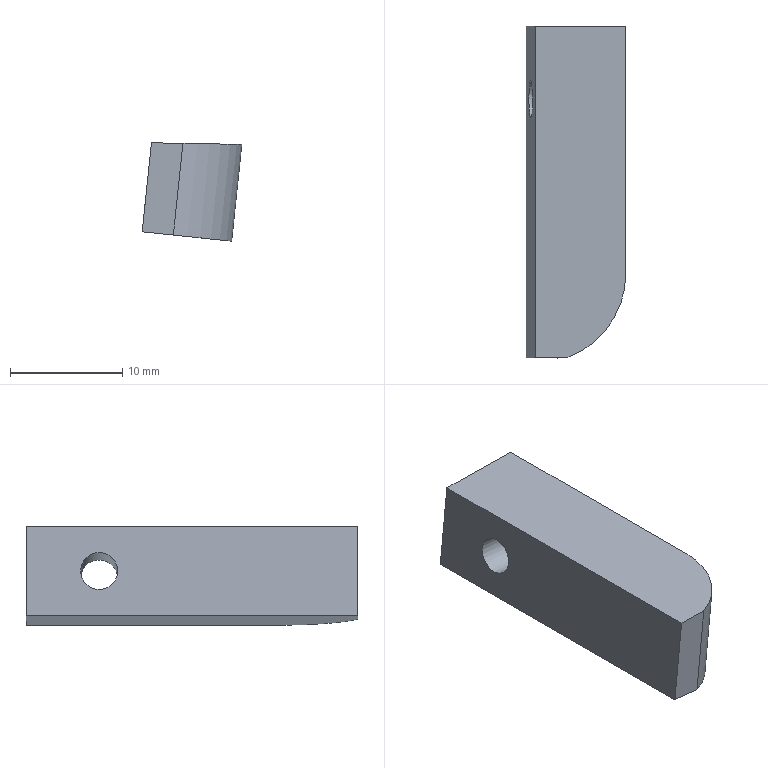Part | STEP file | P011002L001-007 | 1 solid | 9 faces | box 8.861 x 29.5 x 8.749 mm | volume 1779 mm3 | plane 6 | cylinder 2 | cone 1 | commonest cylinder face diameters 3.3 x1 16 x1
STEP:
#1=CARTESIAN_POINT('',(0.,0.,0.));
#2=DIRECTION('',(0.,0.,1.));
#3=DIRECTION('',(1.,0.,0.));
#4=AXIS2_PLACEMENT_3D('',#1,#2,#3);
#5=CARTESIAN_POINT('',(-37.625,-50.96,-34.233));
#6=VERTEX_POINT('',#5);
#7=CARTESIAN_POINT('',(-38.456,-50.96,-42.146));
#8=VERTEX_POINT('',#7);
#9=CARTESIAN_POINT('',(-37.725,-50.96,-35.184));
#10=DIRECTION('',(-0.1045,0.,-0.9945));
#11=VECTOR('',#10,1.);
#12=LINE('',#9,#11);
#13=CARTESIAN_POINT('',(-37.725,-71.46,-35.184));
#14=DIRECTION('',(-0.9945,0.,0.1045));
#15=DIRECTION('',(-0.1045,0.,-0.9945));
#16=AXIS2_PLACEMENT_3D('',#13,#14,#15);
#17=PLANE('',#16);
#18=CARTESIAN_POINT('',(0.,-20.5));
#19=DIRECTION('',(1.,0.));
#20=VECTOR('',#19,1.);
#21=LINE('',#18,#20);
#22=(GEOMETRIC_REPRESENTATION_CONTEXT(2)PARAMETRIC_REPRESENTATION_CONTEXT()REPRESENTATION_CONTEXT('',''));
#23=DEFINITIONAL_REPRESENTATION('',(#21),#22);
#24=PCURVE('',#17,#23);
#25=CARTESIAN_POINT('',(-34.741,-50.96,-35.498));
#26=DIRECTION('',(0.,1.,0.));
#27=DIRECTION('',(0.1045,0.,0.9945));
#28=AXIS2_PLACEMENT_3D('',#25,#26,#27);
#29=PLANE('',#28);
#30=CARTESIAN_POINT('',(0.,-3.));
#31=DIRECTION('',(-1.,0.));
#32=VECTOR('',#31,1.);
#33=LINE('',#30,#32);
#34=(GEOMETRIC_REPRESENTATION_CONTEXT(2)PARAMETRIC_REPRESENTATION_CONTEXT()REPRESENTATION_CONTEXT('',''));
#35=DEFINITIONAL_REPRESENTATION('',(#33),#34);
#36=PCURVE('',#29,#35);
#37=SURFACE_CURVE('',#12,(#24,#36),.PCURVE_S1.);
#38=EDGE_CURVE('',#6,#8,#37,.T.);
#39=ORIENTED_EDGE('',*,*,#38,.T.);
#40=CARTESIAN_POINT('',(-38.456,-80.46,-42.146));
#41=VERTEX_POINT('',#40);
#42=CARTESIAN_POINT('',(-38.456,-71.46,-42.146));
#43=DIRECTION('',(0.,-1.,0.));
#44=VECTOR('',#43,1.);
#45=LINE('',#42,#44);
#46=CARTESIAN_POINT('',(7.,0.));
#47=DIRECTION('',(0.,1.));
#48=VECTOR('',#47,1.);
#49=LINE('',#46,#48);
#50=(GEOMETRIC_REPRESENTATION_CONTEXT(2)PARAMETRIC_REPRESENTATION_CONTEXT()REPRESENTATION_CONTEXT('',''));
#51=DEFINITIONAL_REPRESENTATION('',(#49),#50);
#52=PCURVE('',#17,#51);
#53=CARTESIAN_POINT('',(-35.473,-71.46,-42.46));
#54=DIRECTION('',(-0.1045,0.,-0.9945));
#55=DIRECTION('',(0.9945,0.,-0.1045));
#56=AXIS2_PLACEMENT_3D('',#53,#54,#55);
#57=PLANE('',#56);
#58=CARTESIAN_POINT('',(-3.,0.));
#59=DIRECTION('',(0.,1.));
#60=VECTOR('',#59,1.);
#61=LINE('',#58,#60);
#62=(GEOMETRIC_REPRESENTATION_CONTEXT(2)PARAMETRIC_REPRESENTATION_CONTEXT()REPRESENTATION_CONTEXT('',''));
#63=DEFINITIONAL_REPRESENTATION('',(#61),#62);
#64=PCURVE('',#57,#63);
#65=SURFACE_CURVE('',#45,(#52,#64),.PCURVE_S1.);
#66=EDGE_CURVE('',#8,#41,#65,.T.);
#67=ORIENTED_EDGE('',*,*,#66,.T.);
#68=CARTESIAN_POINT('',(-37.625,-80.46,-34.233));
#69=VERTEX_POINT('',#68);
#70=CARTESIAN_POINT('',(-34.23,-80.46,-1.933));
#71=DIRECTION('',(-0.1045,0.,-0.9945));
#72=VECTOR('',#71,1.);
#73=LINE('',#70,#72);
#74=CARTESIAN_POINT('',(-33.434,9.));
#75=DIRECTION('',(1.,0.));
#76=VECTOR('',#75,1.);
#77=LINE('',#74,#76);
#78=(GEOMETRIC_REPRESENTATION_CONTEXT(2)PARAMETRIC_REPRESENTATION_CONTEXT()REPRESENTATION_CONTEXT('',''));
#79=DEFINITIONAL_REPRESENTATION('',(#77),#78);
#80=PCURVE('',#17,#79);
#81=CARTESIAN_POINT('',(-52.624,-80.46,0.));
#82=DIRECTION('',(0.,-1.,0.));
#83=DIRECTION('',(-1.,0.,0.));
#84=AXIS2_PLACEMENT_3D('',#81,#82,#83);
#85=PLANE('',#84);
#86=CARTESIAN_POINT('',(-18.394,1.933));
#87=DIRECTION('',(0.1045,0.9945));
#88=VECTOR('',#87,1.);
#89=LINE('',#86,#88);
#90=(GEOMETRIC_REPRESENTATION_CONTEXT(2)PARAMETRIC_REPRESENTATION_CONTEXT()REPRESENTATION_CONTEXT('',''));
#91=DEFINITIONAL_REPRESENTATION('',(#89),#90);
#92=PCURVE('',#85,#91);
#93=SURFACE_CURVE('',#73,(#80,#92),.PCURVE_S1.);
#94=EDGE_CURVE('',#69,#41,#93,.T.);
#95=ORIENTED_EDGE('',*,*,#94,.F.);
#96=CARTESIAN_POINT('',(-37.625,-71.46,-34.233));
#97=DIRECTION('',(0.,1.,0.));
#98=VECTOR('',#97,1.);
#99=LINE('',#96,#98);
#100=CARTESIAN_POINT('',(-0.9563,0.));
#101=DIRECTION('',(0.,-1.));
#102=VECTOR('',#101,1.);
#103=LINE('',#100,#102);
#104=(GEOMETRIC_REPRESENTATION_CONTEXT(2)PARAMETRIC_REPRESENTATION_CONTEXT()REPRESENTATION_CONTEXT('',''));
#105=DEFINITIONAL_REPRESENTATION('',(#103),#104);
#106=PCURVE('',#17,#105);
#107=CARTESIAN_POINT('',(-37.123,-71.46,-34.242));
#108=DIRECTION('',(0.01745,0.,0.9998));
#109=DIRECTION('',(0.9998,0.,-0.01745));
#110=AXIS2_PLACEMENT_3D('',#107,#108,#109);
#111=PLANE('',#110);
#112=CARTESIAN_POINT('',(-0.5019,0.));
#113=DIRECTION('',(0.,1.));
#114=VECTOR('',#113,1.);
#115=LINE('',#112,#114);
#116=(GEOMETRIC_REPRESENTATION_CONTEXT(2)PARAMETRIC_REPRESENTATION_CONTEXT()REPRESENTATION_CONTEXT('',''));
#117=DEFINITIONAL_REPRESENTATION('',(#115),#116);
#118=PCURVE('',#111,#117);
#119=SURFACE_CURVE('',#99,(#106,#118),.PCURVE_S1.);
#120=EDGE_CURVE('',#69,#6,#119,.T.);
#121=ORIENTED_EDGE('',*,*,#120,.T.);
#122=EDGE_LOOP('',(#39,#67,#95,#121));
#123=FACE_BOUND('',#122,.T.);
#124=CARTESIAN_POINT('',(-38.211,-57.46,-39.809));
#125=VERTEX_POINT('',#124);
#126=CARTESIAN_POINT('',(-38.038,-57.46,-38.168));
#127=DIRECTION('',(0.9945,0.,-0.1045));
#128=DIRECTION('',(-0.1045,0.,-0.9945));
#129=AXIS2_PLACEMENT_3D('',#126,#127,#128);
#130=CIRCLE('',#129,1.65);
#131=CARTESIAN_POINT('',(4.65,-14.));
#132=CARTESIAN_POINT('',(4.65,-16.858));
#133=CARTESIAN_POINT('',(2.175,-15.429));
#134=CARTESIAN_POINT('',(-0.3,-14.));
#135=CARTESIAN_POINT('',(2.175,-12.571));
#136=CARTESIAN_POINT('',(4.65,-11.142));
#137=CARTESIAN_POINT('',(4.65,-14.));
#138=(BOUNDED_CURVE()B_SPLINE_CURVE(2,(#131,#132,#133,#134,#135,#136,#137),.UNSPECIFIED.,.T.,.F.)B_SPLINE_CURVE_WITH_KNOTS((1,2,2,2,2,1),(-2.094,0.,2.094,4.189,6.283,8.378),.UNSPECIFIED.)CURVE()GEOMETRIC_REPRESENTATION_ITEM()RATIONAL_B_SPLINE_CURVE((1.,0.5,1.,0.5,1.,0.5,1.))REPRESENTATION_ITEM(''));
#139=(GEOMETRIC_REPRESENTATION_CONTEXT(2)PARAMETRIC_REPRESENTATION_CONTEXT()REPRESENTATION_CONTEXT('',''));
#140=DEFINITIONAL_REPRESENTATION('',(#138),#139);
#141=PCURVE('',#17,#140);
#142=CARTESIAN_POINT('',(-31.992,-57.46,-38.803));
#143=DIRECTION('',(-0.9945,0.,0.1045));
#144=DIRECTION('',(0.,-1.,0.));
#145=AXIS2_PLACEMENT_3D('',#142,#143,#144);
#146=CYLINDRICAL_SURFACE('',#145,1.65);
#147=CARTESIAN_POINT('',(10.996,6.08));
#148=DIRECTION('',(-1.,0.));
#149=VECTOR('',#148,1.);
#150=LINE('',#147,#149);
#151=(GEOMETRIC_REPRESENTATION_CONTEXT(2)PARAMETRIC_REPRESENTATION_CONTEXT()REPRESENTATION_CONTEXT('',''));
#152=DEFINITIONAL_REPRESENTATION('',(#150),#151);
#153=PCURVE('',#146,#152);
#154=SURFACE_CURVE('',#130,(#141,#153),.PCURVE_S1.);
#155=EDGE_CURVE('',#125,#125,#154,.T.);
#156=ORIENTED_EDGE('',*,*,#155,.T.);
#157=EDGE_LOOP('',(#156));
#158=FACE_BOUND('',#157,.T.);
#159=ADVANCED_FACE('',(#123,#158),#17,.T.);
#160=CARTESIAN_POINT('',(-30.5,-72.96,-42.982));
#161=VERTEX_POINT('',#160);
#162=CARTESIAN_POINT('',(-30.5,-50.96,-42.982));
#163=VERTEX_POINT('',#162);
#164=CARTESIAN_POINT('',(-30.5,-10.,-42.982));
#165=DIRECTION('',(0.,1.,0.));
#166=VECTOR('',#165,1.);
#167=LINE('',#164,#166);
#168=CARTESIAN_POINT('',(5.,-61.46));
#169=DIRECTION('',(0.,-1.));
#170=VECTOR('',#169,1.);
#171=LINE('',#168,#170);
#172=(GEOMETRIC_REPRESENTATION_CONTEXT(2)PARAMETRIC_REPRESENTATION_CONTEXT()REPRESENTATION_CONTEXT('',''));
#173=DEFINITIONAL_REPRESENTATION('',(#171),#172);
#174=PCURVE('',#57,#173);
#175=CARTESIAN_POINT('',(-27.341,-10.,-12.927));
#176=DIRECTION('',(-0.9945,0.,0.1045));
#177=DIRECTION('',(-0.1045,0.,-0.9945));
#178=AXIS2_PLACEMENT_3D('',#175,#176,#177);
#179=PLANE('',#178);
#180=CARTESIAN_POINT('',(30.221,0.));
#181=DIRECTION('',(0.,-1.));
#182=VECTOR('',#181,1.);
#183=LINE('',#180,#182);
#184=(GEOMETRIC_REPRESENTATION_CONTEXT(2)PARAMETRIC_REPRESENTATION_CONTEXT()REPRESENTATION_CONTEXT('',''));
#185=DEFINITIONAL_REPRESENTATION('',(#183),#184);
#186=PCURVE('',#179,#185);
#187=SURFACE_CURVE('',#167,(#174,#186),.PCURVE_S1.);
#188=EDGE_CURVE('',#161,#163,#187,.T.);
#189=ORIENTED_EDGE('',*,*,#188,.F.);
#190=CARTESIAN_POINT('',(-35.688,-80.46,-42.437));
#191=VERTEX_POINT('',#190);
#192=CARTESIAN_POINT('',(-38.456,-72.96,-42.146));
#193=DIRECTION('',(-0.1045,0.,-0.9945));
#194=DIRECTION('',(-0.9945,0.,0.1045));
#195=AXIS2_PLACEMENT_3D('',#192,#193,#194);
#196=CIRCLE('',#195,8.);
#197=CARTESIAN_POINT('',(-3.,1.5));
#198=DIRECTION('',(-1.,0.));
#199=AXIS2_PLACEMENT_2D('',#197,#198);
#200=CIRCLE('',#199,8.);
#201=(GEOMETRIC_REPRESENTATION_CONTEXT(2)PARAMETRIC_REPRESENTATION_CONTEXT()REPRESENTATION_CONTEXT('',''));
#202=DEFINITIONAL_REPRESENTATION('',(#200),#201);
#203=PCURVE('',#57,#202);
#204=CARTESIAN_POINT('',(-35.298,-72.96,-12.091));
#205=DIRECTION('',(-0.1045,0.,-0.9945));
#206=DIRECTION('',(0.9945,0.,-0.1045));
#207=AXIS2_PLACEMENT_3D('',#204,#205,#206);
#208=CYLINDRICAL_SURFACE('',#207,8.);
#209=CARTESIAN_POINT('',(-3.142,30.221));
#210=DIRECTION('',(1.,-0.000000001));
#211=VECTOR('',#210,1.);
#212=LINE('',#209,#211);
#213=(GEOMETRIC_REPRESENTATION_CONTEXT(2)PARAMETRIC_REPRESENTATION_CONTEXT()REPRESENTATION_CONTEXT('',''));
#214=DEFINITIONAL_REPRESENTATION('',(#212),#213);
#215=PCURVE('',#208,#214);
#216=SURFACE_CURVE('',#196,(#203,#215),.PCURVE_S1.);
#217=EDGE_CURVE('',#161,#191,#216,.T.);
#218=ORIENTED_EDGE('',*,*,#217,.T.);
#219=CARTESIAN_POINT('',(-56.851,-80.46,-40.213));
#220=DIRECTION('',(0.9945,0.,-0.1045));
#221=VECTOR('',#220,1.);
#222=LINE('',#219,#221);
#223=CARTESIAN_POINT('',(-21.495,9.));
#224=DIRECTION('',(1.,0.));
#225=VECTOR('',#224,1.);
#226=LINE('',#223,#225);
#227=(GEOMETRIC_REPRESENTATION_CONTEXT(2)PARAMETRIC_REPRESENTATION_CONTEXT()REPRESENTATION_CONTEXT('',''));
#228=DEFINITIONAL_REPRESENTATION('',(#226),#227);
#229=PCURVE('',#57,#228);
#230=CARTESIAN_POINT('',(4.227,40.213));
#231=DIRECTION('',(-0.9945,0.1045));
#232=VECTOR('',#231,1.);
#233=LINE('',#230,#232);
#234=(GEOMETRIC_REPRESENTATION_CONTEXT(2)PARAMETRIC_REPRESENTATION_CONTEXT()REPRESENTATION_CONTEXT('',''));
#235=DEFINITIONAL_REPRESENTATION('',(#233),#234);
#236=PCURVE('',#85,#235);
#237=SURFACE_CURVE('',#222,(#229,#236),.PCURVE_S1.);
#238=EDGE_CURVE('',#41,#191,#237,.T.);
#239=ORIENTED_EDGE('',*,*,#238,.F.);
#240=ORIENTED_EDGE('',*,*,#66,.F.);
#241=CARTESIAN_POINT('',(-35.473,-50.96,-42.46));
#242=DIRECTION('',(-0.9945,0.,0.1045));
#243=VECTOR('',#242,1.);
#244=LINE('',#241,#243);
#245=CARTESIAN_POINT('',(0.,-20.5));
#246=DIRECTION('',(-1.,0.));
#247=VECTOR('',#246,1.);
#248=LINE('',#245,#247);
#249=(GEOMETRIC_REPRESENTATION_CONTEXT(2)PARAMETRIC_REPRESENTATION_CONTEXT()REPRESENTATION_CONTEXT('',''));
#250=DEFINITIONAL_REPRESENTATION('',(#248),#249);
#251=PCURVE('',#57,#250);
#252=CARTESIAN_POINT('',(-7.,0.));
#253=DIRECTION('',(0.,-1.));
#254=VECTOR('',#253,1.);
#255=LINE('',#252,#254);
#256=(GEOMETRIC_REPRESENTATION_CONTEXT(2)PARAMETRIC_REPRESENTATION_CONTEXT()REPRESENTATION_CONTEXT('',''));
#257=DEFINITIONAL_REPRESENTATION('',(#255),#256);
#258=PCURVE('',#29,#257);
#259=SURFACE_CURVE('',#244,(#251,#258),.PCURVE_S1.);
#260=EDGE_CURVE('',#163,#8,#259,.T.);
#261=ORIENTED_EDGE('',*,*,#260,.F.);
#262=EDGE_LOOP('',(#189,#218,#239,#240,#261));
#263=FACE_BOUND('',#262,.T.);
#264=ADVANCED_FACE('',(#263),#57,.T.);
#265=CARTESIAN_POINT('',(-29.596,-50.96,-34.373));
#266=VERTEX_POINT('',#265);
#267=CARTESIAN_POINT('',(-29.769,-50.96,-36.021));
#268=DIRECTION('',(-0.1045,0.,-0.9945));
#269=VECTOR('',#268,1.);
#270=LINE('',#267,#269);
#271=CARTESIAN_POINT('',(0.000000002,5.));
#272=DIRECTION('',(-1.,0.));
#273=VECTOR('',#272,1.);
#274=LINE('',#271,#273);
#275=(GEOMETRIC_REPRESENTATION_CONTEXT(2)PARAMETRIC_REPRESENTATION_CONTEXT()REPRESENTATION_CONTEXT('',''));
#276=DEFINITIONAL_REPRESENTATION('',(#274),#275);
#277=PCURVE('',#29,#276);
#278=CARTESIAN_POINT('',(23.221,40.96));
#279=DIRECTION('',(1.,0.));
#280=VECTOR('',#279,1.);
#281=LINE('',#278,#280);
#282=(GEOMETRIC_REPRESENTATION_CONTEXT(2)PARAMETRIC_REPRESENTATION_CONTEXT()REPRESENTATION_CONTEXT('',''));
#283=DEFINITIONAL_REPRESENTATION('',(#281),#282);
#284=PCURVE('',#179,#283);
#285=SURFACE_CURVE('',#270,(#277,#284),.PCURVE_S1.);
#286=EDGE_CURVE('',#266,#163,#285,.T.);
#287=ORIENTED_EDGE('',*,*,#286,.T.);
#288=ORIENTED_EDGE('',*,*,#260,.T.);
#289=ORIENTED_EDGE('',*,*,#38,.F.);
#290=CARTESIAN_POINT('',(-34.72,-50.96,-34.284));
#291=DIRECTION('',(0.9998,0.,-0.01745));
#292=VECTOR('',#291,1.);
#293=LINE('',#290,#292);
#294=CARTESIAN_POINT('',(1.209,-0.1058));
#295=DIRECTION('',(0.08716,0.9962));
#296=VECTOR('',#295,1.);
#297=LINE('',#294,#296);
#298=(GEOMETRIC_REPRESENTATION_CONTEXT(2)PARAMETRIC_REPRESENTATION_CONTEXT()REPRESENTATION_CONTEXT('',''));
#299=DEFINITIONAL_REPRESENTATION('',(#297),#298);
#300=PCURVE('',#29,#299);
#301=CARTESIAN_POINT('',(2.403,20.5));
#302=DIRECTION('',(1.,0.));
#303=VECTOR('',#302,1.);
#304=LINE('',#301,#303);
#305=(GEOMETRIC_REPRESENTATION_CONTEXT(2)PARAMETRIC_REPRESENTATION_CONTEXT()REPRESENTATION_CONTEXT('',''));
#306=DEFINITIONAL_REPRESENTATION('',(#304),#305);
#307=PCURVE('',#111,#306);
#308=SURFACE_CURVE('',#293,(#300,#307),.PCURVE_S1.);
#309=EDGE_CURVE('',#6,#266,#308,.T.);
#310=ORIENTED_EDGE('',*,*,#309,.T.);
#311=EDGE_LOOP('',(#287,#288,#289,#310));
#312=FACE_BOUND('',#311,.T.);
#313=ADVANCED_FACE('',(#312),#29,.T.);
#314=ORIENTED_EDGE('',*,*,#238,.T.);
#315=CARTESIAN_POINT('',(-34.831,-80.46,-34.282));
#316=VERTEX_POINT('',#315);
#317=CARTESIAN_POINT('',(-35.24,-80.46,-38.176));
#318=DIRECTION('',(0.1045,0.,0.9945));
#319=VECTOR('',#318,1.);
#320=LINE('',#317,#319);
#321=CARTESIAN_POINT('',(-17.384,38.176));
#322=DIRECTION('',(-0.1045,-0.9945));
#323=VECTOR('',#322,1.);
#324=LINE('',#321,#323);
#325=(GEOMETRIC_REPRESENTATION_CONTEXT(2)PARAMETRIC_REPRESENTATION_CONTEXT()REPRESENTATION_CONTEXT('',''));
#326=DEFINITIONAL_REPRESENTATION('',(#324),#325);
#327=PCURVE('',#85,#326);
#328=CARTESIAN_POINT('',(1.215,25.937));
#329=DIRECTION('',(0.,-1.));
#330=VECTOR('',#329,1.);
#331=LINE('',#328,#330);
#332=(GEOMETRIC_REPRESENTATION_CONTEXT(2)PARAMETRIC_REPRESENTATION_CONTEXT()REPRESENTATION_CONTEXT('',''));
#333=DEFINITIONAL_REPRESENTATION('',(#331),#332);
#334=PCURVE('',#208,#333);
#335=SURFACE_CURVE('',#320,(#327,#334),.PCURVE_S1.);
#336=EDGE_CURVE('',#191,#316,#335,.T.);
#337=ORIENTED_EDGE('',*,*,#336,.T.);
#338=CARTESIAN_POINT('',(-53.217,-80.46,-33.961));
#339=DIRECTION('',(-0.9998,0.,0.01745));
#340=VECTOR('',#339,1.);
#341=LINE('',#338,#340);
#342=CARTESIAN_POINT('',(0.5928,33.961));
#343=DIRECTION('',(0.9998,-0.01745));
#344=VECTOR('',#343,1.);
#345=LINE('',#342,#344);
#346=(GEOMETRIC_REPRESENTATION_CONTEXT(2)PARAMETRIC_REPRESENTATION_CONTEXT()REPRESENTATION_CONTEXT('',''));
#347=DEFINITIONAL_REPRESENTATION('',(#345),#346);
#348=PCURVE('',#85,#347);
#349=CARTESIAN_POINT('',(-16.096,-9.));
#350=DIRECTION('',(-1.,0.));
#351=VECTOR('',#350,1.);
#352=LINE('',#349,#351);
#353=(GEOMETRIC_REPRESENTATION_CONTEXT(2)PARAMETRIC_REPRESENTATION_CONTEXT()REPRESENTATION_CONTEXT('',''));
#354=DEFINITIONAL_REPRESENTATION('',(#352),#353);
#355=PCURVE('',#111,#354);
#356=SURFACE_CURVE('',#341,(#348,#355),.PCURVE_S1.);
#357=EDGE_CURVE('',#316,#69,#356,.T.);
#358=ORIENTED_EDGE('',*,*,#357,.T.);
#359=ORIENTED_EDGE('',*,*,#94,.T.);
#360=EDGE_LOOP('',(#314,#337,#358,#359));
#361=FACE_BOUND('',#360,.T.);
#362=ADVANCED_FACE('',(#361),#85,.T.);
#363=ORIENTED_EDGE('',*,*,#357,.F.);
#364=CARTESIAN_POINT('',(-29.596,-72.96,-34.373));
#365=VERTEX_POINT('',#364);
#366=CARTESIAN_POINT('',(-37.625,-72.96,-34.233));
#367=DIRECTION('',(0.01745,0.,0.9998));
#368=DIRECTION('',(-0.9998,0.,0.01745));
#369=AXIS2_PLACEMENT_3D('',#366,#367,#368);
#370=ELLIPSE('',#369,8.031,8.);
#371=CARTESIAN_POINT('',(-0.5019,-1.5));
#372=DIRECTION('',(-1.,0.));
#373=AXIS2_PLACEMENT_2D('',#371,#372);
#374=ELLIPSE('',#373,8.031,8.);
#375=(GEOMETRIC_REPRESENTATION_CONTEXT(2)PARAMETRIC_REPRESENTATION_CONTEXT()REPRESENTATION_CONTEXT('',''));
#376=DEFINITIONAL_REPRESENTATION('',(#374),#375);
#377=PCURVE('',#111,#376);
#378=CARTESIAN_POINT('',(1.215,22.021));
#379=CARTESIAN_POINT('',(1.197,22.009));
#380=CARTESIAN_POINT('',(1.16,21.985));
#381=CARTESIAN_POINT('',(1.105,21.95));
#382=CARTESIAN_POINT('',(1.05,21.916));
#383=CARTESIAN_POINT('',(0.9944,21.883));
#384=CARTESIAN_POINT('',(0.9392,21.851));
#385=CARTESIAN_POINT('',(0.8839,21.821));
#386=CARTESIAN_POINT('',(0.8287,21.791));
#387=CARTESIAN_POINT('',(0.7734,21.764));
#388=CARTESIAN_POINT('',(0.7182,21.737));
#389=CARTESIAN_POINT('',(0.6629,21.713));
#390=CARTESIAN_POINT('',(0.6077,21.69));
#391=CARTESIAN_POINT('',(0.5524,21.669));
#392=CARTESIAN_POINT('',(0.4972,21.649));
#393=CARTESIAN_POINT('',(0.442,21.632));
#394=CARTESIAN_POINT('',(0.3867,21.616));
#395=CARTESIAN_POINT('',(0.3315,21.603));
#396=CARTESIAN_POINT('',(0.2762,21.591));
#397=CARTESIAN_POINT('',(0.221,21.581));
#398=CARTESIAN_POINT('',(0.1657,21.574));
#399=CARTESIAN_POINT('',(0.1105,21.569));
#400=CARTESIAN_POINT('',(0.05524,21.566));
#401=CARTESIAN_POINT('',(0.01841,21.565));
#402=CARTESIAN_POINT('',(0.,21.565));
#403=B_SPLINE_CURVE_WITH_KNOTS('',3,(#378,#379,#380,#381,#382,#383,#384,#385,#386,#387,#388,#389,#390,#391,#392,#393,#394,#395,#396,#397,#398,#399,#400,#401,#402),.UNSPECIFIED.,.F.,.F.,(4,1,1,1,1,1,1,1,1,1,1,1,1,1,1,1,1,1,1,1,1,1,4),(1.926,1.981,2.037,2.092,2.147,2.202,2.258,2.313,2.368,2.423,2.479,2.534,2.589,2.644,2.7,2.755,2.81,2.865,2.921,2.976,3.031,3.086,3.142),.QUASI_UNIFORM_KNOTS.);
#404=(GEOMETRIC_REPRESENTATION_CONTEXT(2)PARAMETRIC_REPRESENTATION_CONTEXT()REPRESENTATION_CONTEXT('',''));
#405=DEFINITIONAL_REPRESENTATION('',(#403),#404);
#406=PCURVE('',#208,#405);
#407=SURFACE_CURVE('',#370,(#377,#406),.PCURVE_S1.);
#408=EDGE_CURVE('',#316,#365,#407,.T.);
#409=ORIENTED_EDGE('',*,*,#408,.T.);
#410=CARTESIAN_POINT('',(-29.596,-10.,-34.373));
#411=DIRECTION('',(0.,-1.,0.));
#412=VECTOR('',#411,1.);
#413=LINE('',#410,#412);
#414=CARTESIAN_POINT('',(7.529,61.46));
#415=DIRECTION('',(0.,-1.));
#416=VECTOR('',#415,1.);
#417=LINE('',#414,#416);
#418=(GEOMETRIC_REPRESENTATION_CONTEXT(2)PARAMETRIC_REPRESENTATION_CONTEXT()REPRESENTATION_CONTEXT('',''));
#419=DEFINITIONAL_REPRESENTATION('',(#417),#418);
#420=PCURVE('',#111,#419);
#421=CARTESIAN_POINT('',(21.565,0.));
#422=DIRECTION('',(0.,1.));
#423=VECTOR('',#422,1.);
#424=LINE('',#421,#423);
#425=(GEOMETRIC_REPRESENTATION_CONTEXT(2)PARAMETRIC_REPRESENTATION_CONTEXT()REPRESENTATION_CONTEXT('',''));
#426=DEFINITIONAL_REPRESENTATION('',(#424),#425);
#427=PCURVE('',#179,#426);
#428=SURFACE_CURVE('',#413,(#420,#427),.PCURVE_S1.);
#429=EDGE_CURVE('',#266,#365,#428,.T.);
#430=ORIENTED_EDGE('',*,*,#429,.F.);
#431=ORIENTED_EDGE('',*,*,#309,.F.);
#432=ORIENTED_EDGE('',*,*,#120,.F.);
#433=EDGE_LOOP('',(#363,#409,#430,#431,#432));
#434=FACE_BOUND('',#433,.T.);
#435=ADVANCED_FACE('',(#434),#111,.T.);
#436=CARTESIAN_POINT('',(-29.725,-57.46,-35.603));
#437=VERTEX_POINT('',#436);
#438=CARTESIAN_POINT('',(-30.44,-57.46,-42.405));
#439=VERTEX_POINT('',#438);
#440=CARTESIAN_POINT('',(-30.082,-57.46,-39.004));
#441=DIRECTION('',(0.9945,0.,-0.1045));
#442=DIRECTION('',(0.1045,0.,0.9945));
#443=AXIS2_PLACEMENT_3D('',#440,#441,#442);
#444=CIRCLE('',#443,3.42);
#445=CARTESIAN_POINT('',(22.801,47.46));
#446=CARTESIAN_POINT('',(22.801,53.384));
#447=CARTESIAN_POINT('',(27.931,50.422));
#448=CARTESIAN_POINT('',(33.061,47.46));
#449=CARTESIAN_POINT('',(27.931,44.498));
#450=CARTESIAN_POINT('',(22.801,41.536));
#451=CARTESIAN_POINT('',(22.801,47.46));
#452=(BOUNDED_CURVE()B_SPLINE_CURVE(2,(#445,#446,#447,#448,#449,#450,#451),.UNSPECIFIED.,.T.,.F.)B_SPLINE_CURVE_WITH_KNOTS((1,2,2,2,2,1),(-2.094,0.,2.094,4.189,6.283,8.378),.UNSPECIFIED.)CURVE()GEOMETRIC_REPRESENTATION_ITEM()RATIONAL_B_SPLINE_CURVE((1.,0.5,1.,0.5,1.,0.5,1.))REPRESENTATION_ITEM(''));
#453=(GEOMETRIC_REPRESENTATION_CONTEXT(2)PARAMETRIC_REPRESENTATION_CONTEXT()REPRESENTATION_CONTEXT('',''));
#454=DEFINITIONAL_REPRESENTATION('',(#452),#453);
#455=PCURVE('',#179,#454);
#456=CARTESIAN_POINT('',(-31.992,-57.46,-38.803));
#457=DIRECTION('',(0.9945,0.,-0.1045));
#458=DIRECTION('',(0.,-1.,0.));
#459=AXIS2_PLACEMENT_3D('',#456,#457,#458);
#460=CONICAL_SURFACE('',#459,1.5,0.7854);
#461=CARTESIAN_POINT('',(4.712,1.92));
#462=DIRECTION('',(1.,0.));
#463=VECTOR('',#462,1.);
#464=LINE('',#461,#463);
#465=(GEOMETRIC_REPRESENTATION_CONTEXT(2)PARAMETRIC_REPRESENTATION_CONTEXT()REPRESENTATION_CONTEXT('',''));
#466=DEFINITIONAL_REPRESENTATION('',(#464),#465);
#467=PCURVE('',#460,#466);
#468=SURFACE_CURVE('',#444,(#455,#467),.PCURVE_S1.);
#469=EDGE_CURVE('',#437,#439,#468,.T.);
#470=ORIENTED_EDGE('',*,*,#469,.F.);
#471=CARTESIAN_POINT('',(-30.082,-57.46,-39.004));
#472=DIRECTION('',(0.9945,0.,-0.1045));
#473=DIRECTION('',(0.1045,0.,0.9945));
#474=AXIS2_PLACEMENT_3D('',#471,#472,#473);
#475=CIRCLE('',#474,3.42);
#476=CARTESIAN_POINT('',(22.801,47.46));
#477=CARTESIAN_POINT('',(22.801,53.384));
#478=CARTESIAN_POINT('',(27.931,50.422));
#479=CARTESIAN_POINT('',(33.061,47.46));
#480=CARTESIAN_POINT('',(27.931,44.498));
#481=CARTESIAN_POINT('',(22.801,41.536));
#482=CARTESIAN_POINT('',(22.801,47.46));
#483=(BOUNDED_CURVE()B_SPLINE_CURVE(2,(#476,#477,#478,#479,#480,#481,#482),.UNSPECIFIED.,.T.,.F.)B_SPLINE_CURVE_WITH_KNOTS((1,2,2,2,2,1),(-2.094,0.,2.094,4.189,6.283,8.378),.UNSPECIFIED.)CURVE()GEOMETRIC_REPRESENTATION_ITEM()RATIONAL_B_SPLINE_CURVE((1.,0.5,1.,0.5,1.,0.5,1.))REPRESENTATION_ITEM(''));
#484=(GEOMETRIC_REPRESENTATION_CONTEXT(2)PARAMETRIC_REPRESENTATION_CONTEXT()REPRESENTATION_CONTEXT('',''));
#485=DEFINITIONAL_REPRESENTATION('',(#483),#484);
#486=PCURVE('',#179,#485);
#487=CARTESIAN_POINT('',(-1.571,1.92));
#488=DIRECTION('',(1.,0.));
#489=VECTOR('',#488,1.);
#490=LINE('',#487,#489);
#491=(GEOMETRIC_REPRESENTATION_CONTEXT(2)PARAMETRIC_REPRESENTATION_CONTEXT()REPRESENTATION_CONTEXT('',''));
#492=DEFINITIONAL_REPRESENTATION('',(#490),#491);
#493=PCURVE('',#460,#492);
#494=SURFACE_CURVE('',#475,(#486,#493),.PCURVE_S1.);
#495=EDGE_CURVE('',#439,#437,#494,.T.);
#496=ORIENTED_EDGE('',*,*,#495,.F.);
#497=EDGE_LOOP('',(#470,#496));
#498=FACE_BOUND('',#497,.T.);
#499=ORIENTED_EDGE('',*,*,#429,.T.);
#500=CARTESIAN_POINT('',(-30.048,-72.96,-38.678));
#501=DIRECTION('',(-0.1045,0.,-0.9945));
#502=VECTOR('',#501,1.);
#503=LINE('',#500,#502);
#504=CARTESIAN_POINT('',(25.893,62.96));
#505=DIRECTION('',(1.,0.));
#506=VECTOR('',#505,1.);
#507=LINE('',#504,#506);
#508=(GEOMETRIC_REPRESENTATION_CONTEXT(2)PARAMETRIC_REPRESENTATION_CONTEXT()REPRESENTATION_CONTEXT('',''));
#509=DEFINITIONAL_REPRESENTATION('',(#507),#508);
#510=PCURVE('',#179,#509);
#511=CARTESIAN_POINT('',(0.,25.893));
#512=DIRECTION('',(0.,1.));
#513=VECTOR('',#512,1.);
#514=LINE('',#511,#513);
#515=(GEOMETRIC_REPRESENTATION_CONTEXT(2)PARAMETRIC_REPRESENTATION_CONTEXT()REPRESENTATION_CONTEXT('',''));
#516=DEFINITIONAL_REPRESENTATION('',(#514),#515);
#517=PCURVE('',#208,#516);
#518=SURFACE_CURVE('',#503,(#510,#517),.PCURVE_S1.);
#519=EDGE_CURVE('',#365,#161,#518,.T.);
#520=ORIENTED_EDGE('',*,*,#519,.T.);
#521=ORIENTED_EDGE('',*,*,#188,.T.);
#522=ORIENTED_EDGE('',*,*,#286,.F.);
#523=EDGE_LOOP('',(#499,#520,#521,#522));
#524=FACE_BOUND('',#523,.T.);
#525=ADVANCED_FACE('',(#498,#524),#179,.F.);
#526=ORIENTED_EDGE('',*,*,#408,.F.);
#527=ORIENTED_EDGE('',*,*,#336,.F.);
#528=ORIENTED_EDGE('',*,*,#217,.F.);
#529=ORIENTED_EDGE('',*,*,#519,.F.);
#530=EDGE_LOOP('',(#526,#527,#528,#529));
#531=FACE_BOUND('',#530,.T.);
#532=ADVANCED_FACE('',(#531),#208,.T.);
#533=ORIENTED_EDGE('',*,*,#155,.T.);
#534=CARTESIAN_POINT('',(-32.015,-57.46,-40.46));
#535=VERTEX_POINT('',#534);
#536=CARTESIAN_POINT('',(-32.015,-57.46,-40.46));
#537=CARTESIAN_POINT('',(-38.211,-57.46,-39.809));
#538=B_SPLINE_CURVE_WITH_KNOTS('',1,(#536,#537),.UNSPECIFIED.,.F.,.F.,(2,2),(-0.15,6.08),.PIECEWISE_BEZIER_KNOTS.);
#539=CARTESIAN_POINT('',(4.712,0.));
#540=DIRECTION('',(0.,1.));
#541=VECTOR('',#540,1.);
#542=LINE('',#539,#541);
#543=(GEOMETRIC_REPRESENTATION_CONTEXT(2)PARAMETRIC_REPRESENTATION_CONTEXT()REPRESENTATION_CONTEXT('',''));
#544=DEFINITIONAL_REPRESENTATION('',(#542),#543);
#545=PCURVE('',#146,#544);
#546=CARTESIAN_POINT('',(10.996,0.));
#547=DIRECTION('',(0.,1.));
#548=VECTOR('',#547,1.);
#549=LINE('',#546,#548);
#550=(GEOMETRIC_REPRESENTATION_CONTEXT(2)PARAMETRIC_REPRESENTATION_CONTEXT()REPRESENTATION_CONTEXT('',''));
#551=DEFINITIONAL_REPRESENTATION('',(#549),#550);
#552=PCURVE('',#146,#551);
#553=SEAM_CURVE('',#538,(#545,#552),.PCURVE_S1.);
#554=EDGE_CURVE('',#535,#125,#553,.T.);
#555=ORIENTED_EDGE('',*,*,#554,.F.);
#556=CARTESIAN_POINT('',(-31.843,-55.81,-38.819));
#557=VERTEX_POINT('',#556);
#558=CARTESIAN_POINT('',(-31.843,-57.46,-38.819));
#559=DIRECTION('',(0.9945,0.,-0.1045));
#560=DIRECTION('',(0.,1.,0.));
#561=AXIS2_PLACEMENT_3D('',#558,#559,#560);
#562=CIRCLE('',#561,1.65);
#563=CARTESIAN_POINT('',(9.425,-0.15));
#564=DIRECTION('',(-1.,0.));
#565=VECTOR('',#564,1.);
#566=LINE('',#563,#565);
#567=(GEOMETRIC_REPRESENTATION_CONTEXT(2)PARAMETRIC_REPRESENTATION_CONTEXT()REPRESENTATION_CONTEXT('',''));
#568=DEFINITIONAL_REPRESENTATION('',(#566),#567);
#569=PCURVE('',#146,#568);
#570=CARTESIAN_POINT('',(3.142,0.15));
#571=DIRECTION('',(1.,0.));
#572=VECTOR('',#571,1.);
#573=LINE('',#570,#572);
#574=(GEOMETRIC_REPRESENTATION_CONTEXT(2)PARAMETRIC_REPRESENTATION_CONTEXT()REPRESENTATION_CONTEXT('',''));
#575=DEFINITIONAL_REPRESENTATION('',(#573),#574);
#576=PCURVE('',#460,#575);
#577=SURFACE_CURVE('',#562,(#569,#576),.PCURVE_S1.);
#578=EDGE_CURVE('',#557,#535,#577,.T.);
#579=ORIENTED_EDGE('',*,*,#578,.F.);
#580=CARTESIAN_POINT('',(-31.843,-57.46,-38.819));
#581=DIRECTION('',(0.9945,0.,-0.1045));
#582=DIRECTION('',(0.,1.,0.));
#583=AXIS2_PLACEMENT_3D('',#580,#581,#582);
#584=CIRCLE('',#583,1.65);
#585=CARTESIAN_POINT('',(15.708,-0.15));
#586=DIRECTION('',(-1.,0.));
#587=VECTOR('',#586,1.);
#588=LINE('',#585,#587);
#589=(GEOMETRIC_REPRESENTATION_CONTEXT(2)PARAMETRIC_REPRESENTATION_CONTEXT()REPRESENTATION_CONTEXT('',''));
#590=DEFINITIONAL_REPRESENTATION('',(#588),#589);
#591=PCURVE('',#146,#590);
#592=CARTESIAN_POINT('',(-3.142,0.15));
#593=DIRECTION('',(1.,0.));
#594=VECTOR('',#593,1.);
#595=LINE('',#592,#594);
#596=(GEOMETRIC_REPRESENTATION_CONTEXT(2)PARAMETRIC_REPRESENTATION_CONTEXT()REPRESENTATION_CONTEXT('',''));
#597=DEFINITIONAL_REPRESENTATION('',(#595),#596);
#598=PCURVE('',#460,#597);
#599=SURFACE_CURVE('',#584,(#591,#598),.PCURVE_S1.);
#600=EDGE_CURVE('',#535,#557,#599,.T.);
#601=ORIENTED_EDGE('',*,*,#600,.F.);
#602=ORIENTED_EDGE('',*,*,#554,.T.);
#603=EDGE_LOOP('',(#533,#555,#579,#601,#602));
#604=FACE_BOUND('',#603,.F.);
#605=ADVANCED_FACE('',(#604),#146,.F.);
#606=ORIENTED_EDGE('',*,*,#600,.T.);
#607=ORIENTED_EDGE('',*,*,#578,.T.);
#608=CARTESIAN_POINT('',(-32.015,-57.46,-40.46));
#609=CARTESIAN_POINT('',(-30.44,-57.46,-42.405));
#610=B_SPLINE_CURVE_WITH_KNOTS('',1,(#608,#609),.UNSPECIFIED.,.F.,.F.,(2,2),(0.2121,2.715),.PIECEWISE_BEZIER_KNOTS.);
#611=CARTESIAN_POINT('',(7.854,0.));
#612=DIRECTION('',(0.,1.));
#613=VECTOR('',#612,1.);
#614=LINE('',#611,#613);
#615=(GEOMETRIC_REPRESENTATION_CONTEXT(2)PARAMETRIC_REPRESENTATION_CONTEXT()REPRESENTATION_CONTEXT('',''));
#616=DEFINITIONAL_REPRESENTATION('',(#614),#615);
#617=PCURVE('',#460,#616);
#618=CARTESIAN_POINT('',(1.571,0.));
#619=DIRECTION('',(0.,1.));
#620=VECTOR('',#619,1.);
#621=LINE('',#618,#620);
#622=(GEOMETRIC_REPRESENTATION_CONTEXT(2)PARAMETRIC_REPRESENTATION_CONTEXT()REPRESENTATION_CONTEXT('',''));
#623=DEFINITIONAL_REPRESENTATION('',(#621),#622);
#624=PCURVE('',#460,#623);
#625=SEAM_CURVE('',#610,(#617,#624),.PCURVE_S1.);
#626=EDGE_CURVE('',#535,#439,#625,.T.);
#627=ORIENTED_EDGE('',*,*,#626,.T.);
#628=ORIENTED_EDGE('',*,*,#469,.F.);
#629=ORIENTED_EDGE('',*,*,#495,.F.);
#630=ORIENTED_EDGE('',*,*,#626,.F.);
#631=EDGE_LOOP('',(#606,#607,#627,#628,#629,#630));
#632=FACE_BOUND('',#631,.F.);
#633=ADVANCED_FACE('',(#632),#460,.F.);
#634=CLOSED_SHELL('',(#159,#264,#313,#362,#435,#525,#532,#605,#633));
#635=MANIFOLD_SOLID_BREP('',#634);
#636=(LENGTH_UNIT()NAMED_UNIT(*)SI_UNIT(.MILLI.,.METRE.));
#637=UNCERTAINTY_MEASURE_WITH_UNIT(LENGTH_MEASURE(0.000002),#636,'','');
#638=(NAMED_UNIT(*)PLANE_ANGLE_UNIT()SI_UNIT($,.RADIAN.));
#639=(NAMED_UNIT(*)SI_UNIT($,.STERADIAN.)SOLID_ANGLE_UNIT());
#640=(GEOMETRIC_REPRESENTATION_CONTEXT(3)GLOBAL_UNCERTAINTY_ASSIGNED_CONTEXT((#637))GLOBAL_UNIT_ASSIGNED_CONTEXT((#636,#638,#639))REPRESENTATION_CONTEXT('',''));
#641=ADVANCED_BREP_SHAPE_REPRESENTATION('',(#4,#635),#640);